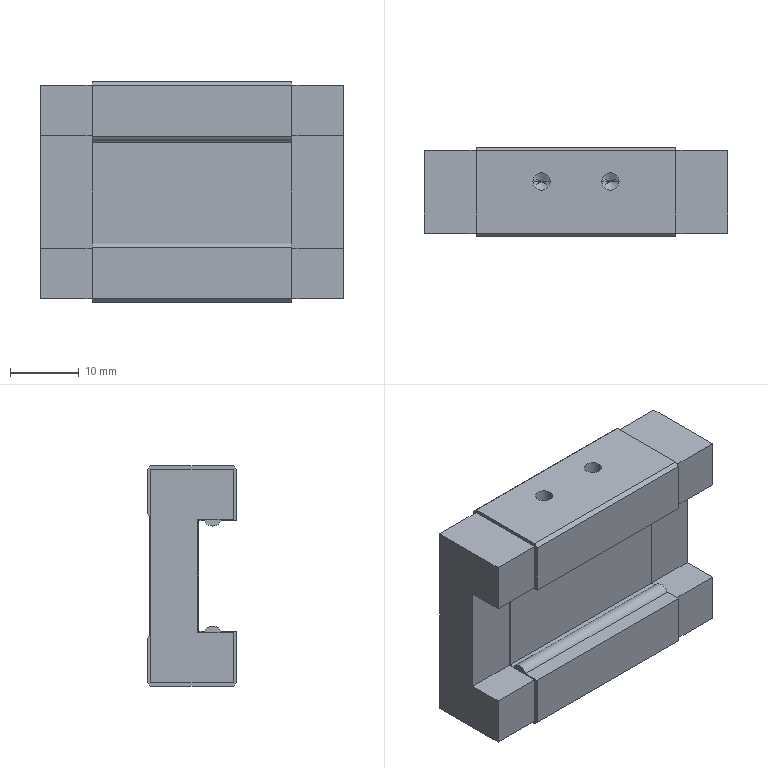Part | NX | 1 solid | 73 faces | box 44 x 13 x 32 mm | volume 13440 mm3 | plane 38 | cylinder 19 | cone 16 | commonest cylinder face diameters 2.5 x8 3.3 x8 2.7 x3